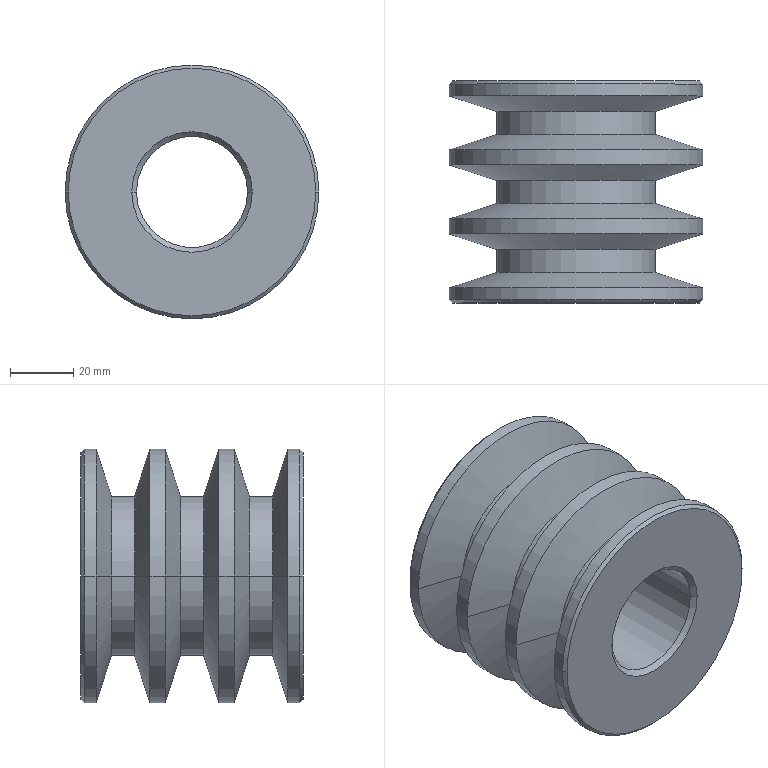Part | Creo | features DATUM PLANE 3, CHAMFER 2, COORDINATE SYSTEM 1, CURVE 1, PROTRUSION 1 | 1 solid | 38 faces | box 80 x 70 x 80 mm | volume 169146 mm3 | cone 20 | cylinder 16 | plane 2 | commonest cylinder face diameters 80 x8 50.008 x6 35 x2
STEP:
#1=CARTESIAN_POINT('',(0.,0.,0.));
#2=DIRECTION('',(0.,0.,1.));
#3=DIRECTION('',(1.,0.,0.));
#4=AXIS2_PLACEMENT_3D('',#1,#2,#3);
#5=CARTESIAN_POINT('',(39.,70.,0.));
#6=VERTEX_POINT('',#5);
#7=CARTESIAN_POINT('',(-39.,70.,0.));
#8=VERTEX_POINT('',#7);
#9=CARTESIAN_POINT('',(0.,70.,0.));
#10=DIRECTION('',(0.,1.,0.));
#11=DIRECTION('',(1.,0.,0.));
#12=AXIS2_PLACEMENT_3D('',#9,#10,#11);
#13=CIRCLE('',#12,39.);
#14=EDGE_CURVE('',#6,#8,#13,.T.);
#15=ORIENTED_EDGE('',*,*,#14,.F.);
#16=CARTESIAN_POINT('',(0.,70.,0.));
#17=DIRECTION('',(0.,1.,0.));
#18=DIRECTION('',(-1.,0.,0.));
#19=AXIS2_PLACEMENT_3D('',#16,#17,#18);
#20=CIRCLE('',#19,39.);
#21=EDGE_CURVE('',#8,#6,#20,.T.);
#22=ORIENTED_EDGE('',*,*,#21,.F.);
#23=EDGE_LOOP('',(#15,#22));
#24=FACE_OUTER_BOUND('',#23,.F.);
#25=CARTESIAN_POINT('',(-19.,70.,0.));
#26=VERTEX_POINT('',#25);
#27=CARTESIAN_POINT('',(19.,70.,0.));
#28=VERTEX_POINT('',#27);
#29=CARTESIAN_POINT('',(0.,70.,0.));
#30=DIRECTION('',(0.,1.,0.));
#31=DIRECTION('',(-1.,0.,0.));
#32=AXIS2_PLACEMENT_3D('',#29,#30,#31);
#33=CIRCLE('',#32,19.);
#34=EDGE_CURVE('',#26,#28,#33,.T.);
#35=ORIENTED_EDGE('',*,*,#34,.T.);
#36=CARTESIAN_POINT('',(0.,70.,0.));
#37=DIRECTION('',(0.,1.,0.));
#38=DIRECTION('',(1.,0.,0.));
#39=AXIS2_PLACEMENT_3D('',#36,#37,#38);
#40=CIRCLE('',#39,19.);
#41=EDGE_CURVE('',#28,#26,#40,.T.);
#42=ORIENTED_EDGE('',*,*,#41,.T.);
#43=EDGE_LOOP('',(#35,#42));
#44=FACE_BOUND('',#43,.F.);
#45=CARTESIAN_POINT('',(0.,70.,0.));
#46=DIRECTION('',(0.,1.,0.));
#47=DIRECTION('',(1.,0.,0.));
#48=AXIS2_PLACEMENT_3D('',#45,#46,#47);
#49=PLANE('',#48);
#50=ADVANCED_FACE('',(#24,#44),#49,.T.);
#51=CARTESIAN_POINT('',(-17.5,68.5,0.));
#52=VERTEX_POINT('',#51);
#53=CARTESIAN_POINT('',(17.5,68.5,0.));
#54=VERTEX_POINT('',#53);
#55=CARTESIAN_POINT('',(0.,68.5,0.));
#56=DIRECTION('',(0.,1.,0.));
#57=DIRECTION('',(-1.,0.,0.));
#58=AXIS2_PLACEMENT_3D('',#55,#56,#57);
#59=CIRCLE('',#58,17.5);
#60=EDGE_CURVE('',#52,#54,#59,.T.);
#61=ORIENTED_EDGE('',*,*,#60,.T.);
#62=CARTESIAN_POINT('',(17.5,68.5,0.000000002));
#63=DIRECTION('',(0.7071,0.7071,0.000000001));
#64=VECTOR('',#63,2.121);
#65=LINE('',#62,#64);
#66=EDGE_CURVE('',#54,#28,#65,.T.);
#67=ORIENTED_EDGE('',*,*,#66,.T.);
#68=ORIENTED_EDGE('',*,*,#34,.F.);
#69=CARTESIAN_POINT('',(-17.5,68.5,-0.000000002));
#70=DIRECTION('',(-0.7071,0.7071,-0.000000001));
#71=VECTOR('',#70,2.121);
#72=LINE('',#69,#71);
#73=EDGE_CURVE('',#52,#26,#72,.T.);
#74=ORIENTED_EDGE('',*,*,#73,.F.);
#75=EDGE_LOOP('',(#61,#67,#68,#74));
#76=FACE_OUTER_BOUND('',#75,.F.);
#77=CARTESIAN_POINT('',(0.,69.25,0.));
#78=DIRECTION('',(0.,1.,0.));
#79=DIRECTION('',(0.,0.,-1.));
#80=AXIS2_PLACEMENT_3D('',#77,#78,#79);
#81=CONICAL_SURFACE('',#80,18.25,45.);
#82=ADVANCED_FACE('',(#76),#81,.F.);
#83=ORIENTED_EDGE('',*,*,#60,.F.);
#84=CARTESIAN_POINT('',(-17.5,1.5,0.));
#85=VERTEX_POINT('',#84);
#86=CARTESIAN_POINT('',(-17.5,68.5,-0.000000002));
#87=DIRECTION('',(0.,-1.,0.));
#88=VECTOR('',#87,67.);
#89=LINE('',#86,#88);
#90=EDGE_CURVE('',#52,#85,#89,.T.);
#91=ORIENTED_EDGE('',*,*,#90,.T.);
#92=CARTESIAN_POINT('',(17.5,1.5,0.));
#93=VERTEX_POINT('',#92);
#94=CARTESIAN_POINT('',(0.,1.5,0.));
#95=DIRECTION('',(0.,1.,0.));
#96=DIRECTION('',(-1.,0.,0.));
#97=AXIS2_PLACEMENT_3D('',#94,#95,#96);
#98=CIRCLE('',#97,17.5);
#99=EDGE_CURVE('',#85,#93,#98,.T.);
#100=ORIENTED_EDGE('',*,*,#99,.T.);
#101=CARTESIAN_POINT('',(17.5,68.5,0.000000002));
#102=DIRECTION('',(0.,-1.,0.));
#103=VECTOR('',#102,67.);
#104=LINE('',#101,#103);
#105=EDGE_CURVE('',#54,#93,#104,.T.);
#106=ORIENTED_EDGE('',*,*,#105,.F.);
#107=EDGE_LOOP('',(#83,#91,#100,#106));
#108=FACE_OUTER_BOUND('',#107,.F.);
#109=CARTESIAN_POINT('',(0.,0.,0.));
#110=DIRECTION('',(0.,1.,0.));
#111=DIRECTION('',(1.,0.,0.));
#112=AXIS2_PLACEMENT_3D('',#109,#110,#111);
#113=CYLINDRICAL_SURFACE('',#112,17.5);
#114=ADVANCED_FACE('',(#108),#113,.F.);
#115=CARTESIAN_POINT('',(0.,68.5,0.));
#116=DIRECTION('',(0.,1.,0.));
#117=DIRECTION('',(1.,0.,0.));
#118=AXIS2_PLACEMENT_3D('',#115,#116,#117);
#119=CIRCLE('',#118,17.5);
#120=EDGE_CURVE('',#54,#52,#119,.T.);
#121=ORIENTED_EDGE('',*,*,#120,.F.);
#122=ORIENTED_EDGE('',*,*,#105,.T.);
#123=CARTESIAN_POINT('',(0.,1.5,0.));
#124=DIRECTION('',(0.,1.,0.));
#125=DIRECTION('',(1.,0.,0.));
#126=AXIS2_PLACEMENT_3D('',#123,#124,#125);
#127=CIRCLE('',#126,17.5);
#128=EDGE_CURVE('',#93,#85,#127,.T.);
#129=ORIENTED_EDGE('',*,*,#128,.T.);
#130=ORIENTED_EDGE('',*,*,#90,.F.);
#131=EDGE_LOOP('',(#121,#122,#129,#130));
#132=FACE_OUTER_BOUND('',#131,.F.);
#133=CARTESIAN_POINT('',(0.,0.,0.));
#134=DIRECTION('',(0.,1.,0.));
#135=DIRECTION('',(1.,0.,0.));
#136=AXIS2_PLACEMENT_3D('',#133,#134,#135);
#137=CYLINDRICAL_SURFACE('',#136,17.5);
#138=ADVANCED_FACE('',(#132),#137,.F.);
#139=ORIENTED_EDGE('',*,*,#120,.T.);
#140=ORIENTED_EDGE('',*,*,#73,.T.);
#141=ORIENTED_EDGE('',*,*,#41,.F.);
#142=ORIENTED_EDGE('',*,*,#66,.F.);
#143=EDGE_LOOP('',(#139,#140,#141,#142));
#144=FACE_OUTER_BOUND('',#143,.F.);
#145=CARTESIAN_POINT('',(0.,69.25,0.));
#146=DIRECTION('',(0.,1.,0.));
#147=DIRECTION('',(0.,0.,-1.));
#148=AXIS2_PLACEMENT_3D('',#145,#146,#147);
#149=CONICAL_SURFACE('',#148,18.25,45.);
#150=ADVANCED_FACE('',(#144),#149,.F.);
#151=CARTESIAN_POINT('',(19.,0.,0.));
#152=VERTEX_POINT('',#151);
#153=CARTESIAN_POINT('',(-19.,0.,0.));
#154=VERTEX_POINT('',#153);
#155=CARTESIAN_POINT('',(0.,0.,0.));
#156=DIRECTION('',(0.,1.,0.));
#157=DIRECTION('',(1.,0.,0.));
#158=AXIS2_PLACEMENT_3D('',#155,#156,#157);
#159=CIRCLE('',#158,19.);
#160=EDGE_CURVE('',#152,#154,#159,.T.);
#161=ORIENTED_EDGE('',*,*,#160,.T.);
#162=CARTESIAN_POINT('',(-19.,0.000000002,0.000000012));
#163=DIRECTION('',(0.7071,0.7071,-0.000000002));
#164=VECTOR('',#163,2.121);
#165=LINE('',#162,#164);
#166=EDGE_CURVE('',#154,#85,#165,.T.);
#167=ORIENTED_EDGE('',*,*,#166,.T.);
#168=ORIENTED_EDGE('',*,*,#128,.F.);
#169=CARTESIAN_POINT('',(19.,0.000000002,-0.000000012));
#170=DIRECTION('',(-0.7071,0.7071,0.000000002));
#171=VECTOR('',#170,2.121);
#172=LINE('',#169,#171);
#173=EDGE_CURVE('',#152,#93,#172,.T.);
#174=ORIENTED_EDGE('',*,*,#173,.F.);
#175=EDGE_LOOP('',(#161,#167,#168,#174));
#176=FACE_OUTER_BOUND('',#175,.F.);
#177=CARTESIAN_POINT('',(0.,0.75,0.));
#178=DIRECTION('',(0.,-1.,0.));
#179=DIRECTION('',(0.,0.,-1.));
#180=AXIS2_PLACEMENT_3D('',#177,#178,#179);
#181=CONICAL_SURFACE('',#180,18.25,45.);
#182=ADVANCED_FACE('',(#176),#181,.F.);
#183=CARTESIAN_POINT('',(39.,0.,0.));
#184=VERTEX_POINT('',#183);
#185=CARTESIAN_POINT('',(-39.,0.,0.));
#186=VERTEX_POINT('',#185);
#187=CARTESIAN_POINT('',(0.,0.,0.));
#188=DIRECTION('',(0.,1.,0.));
#189=DIRECTION('',(1.,0.,0.));
#190=AXIS2_PLACEMENT_3D('',#187,#188,#189);
#191=CIRCLE('',#190,39.);
#192=EDGE_CURVE('',#184,#186,#191,.T.);
#193=ORIENTED_EDGE('',*,*,#192,.T.);
#194=CARTESIAN_POINT('',(0.,0.,0.));
#195=DIRECTION('',(0.,1.,0.));
#196=DIRECTION('',(-1.,0.,0.));
#197=AXIS2_PLACEMENT_3D('',#194,#195,#196);
#198=CIRCLE('',#197,39.);
#199=EDGE_CURVE('',#186,#184,#198,.T.);
#200=ORIENTED_EDGE('',*,*,#199,.T.);
#201=EDGE_LOOP('',(#193,#200));
#202=FACE_OUTER_BOUND('',#201,.F.);
#203=CARTESIAN_POINT('',(0.,0.,0.));
#204=DIRECTION('',(0.,1.,0.));
#205=DIRECTION('',(-1.,0.,0.));
#206=AXIS2_PLACEMENT_3D('',#203,#204,#205);
#207=CIRCLE('',#206,19.);
#208=EDGE_CURVE('',#154,#152,#207,.T.);
#209=ORIENTED_EDGE('',*,*,#208,.F.);
#210=ORIENTED_EDGE('',*,*,#160,.F.);
#211=EDGE_LOOP('',(#209,#210));
#212=FACE_BOUND('',#211,.F.);
#213=CARTESIAN_POINT('',(0.,0.,0.));
#214=DIRECTION('',(0.,1.,0.));
#215=DIRECTION('',(1.,0.,0.));
#216=AXIS2_PLACEMENT_3D('',#213,#214,#215);
#217=PLANE('',#216);
#218=ADVANCED_FACE('',(#202,#212),#217,.F.);
#219=ORIENTED_EDGE('',*,*,#208,.T.);
#220=ORIENTED_EDGE('',*,*,#173,.T.);
#221=ORIENTED_EDGE('',*,*,#99,.F.);
#222=ORIENTED_EDGE('',*,*,#166,.F.);
#223=EDGE_LOOP('',(#219,#220,#221,#222));
#224=FACE_OUTER_BOUND('',#223,.F.);
#225=CARTESIAN_POINT('',(0.,0.75,0.));
#226=DIRECTION('',(0.,-1.,0.));
#227=DIRECTION('',(0.,0.,-1.));
#228=AXIS2_PLACEMENT_3D('',#225,#226,#227);
#229=CONICAL_SURFACE('',#228,18.25,45.);
#230=ADVANCED_FACE('',(#224),#229,.F.);
#231=CARTESIAN_POINT('',(40.,1.,0.));
#232=VERTEX_POINT('',#231);
#233=CARTESIAN_POINT('',(-40.,1.,0.));
#234=VERTEX_POINT('',#233);
#235=CARTESIAN_POINT('',(0.,1.,0.));
#236=DIRECTION('',(0.,1.,0.));
#237=DIRECTION('',(1.,0.,0.));
#238=AXIS2_PLACEMENT_3D('',#235,#236,#237);
#239=CIRCLE('',#238,40.);
#240=EDGE_CURVE('',#232,#234,#239,.T.);
#241=ORIENTED_EDGE('',*,*,#240,.T.);
#242=CARTESIAN_POINT('',(-40.,1.,-0.000000001));
#243=DIRECTION('',(0.7071,-0.7071,0.));
#244=VECTOR('',#243,1.414);
#245=LINE('',#242,#244);
#246=EDGE_CURVE('',#234,#186,#245,.T.);
#247=ORIENTED_EDGE('',*,*,#246,.T.);
#248=ORIENTED_EDGE('',*,*,#192,.F.);
#249=CARTESIAN_POINT('',(40.,1.,0.000000001));
#250=DIRECTION('',(-0.7071,-0.7071,0.));
#251=VECTOR('',#250,1.414);
#252=LINE('',#249,#251);
#253=EDGE_CURVE('',#232,#184,#252,.T.);
#254=ORIENTED_EDGE('',*,*,#253,.F.);
#255=EDGE_LOOP('',(#241,#247,#248,#254));
#256=FACE_OUTER_BOUND('',#255,.F.);
#257=CARTESIAN_POINT('',(0.,0.5,0.));
#258=DIRECTION('',(0.,1.,0.));
#259=DIRECTION('',(0.,0.,-1.));
#260=AXIS2_PLACEMENT_3D('',#257,#258,#259);
#261=CONICAL_SURFACE('',#260,39.5,45.);
#262=ADVANCED_FACE('',(#256),#261,.T.);
#263=ORIENTED_EDGE('',*,*,#240,.F.);
#264=CARTESIAN_POINT('',(40.,4.751,0.));
#265=VERTEX_POINT('',#264);
#266=CARTESIAN_POINT('',(40.,1.,0.000000001));
#267=DIRECTION('',(0.,1.,0.));
#268=VECTOR('',#267,3.751);
#269=LINE('',#266,#268);
#270=EDGE_CURVE('',#232,#265,#269,.T.);
#271=ORIENTED_EDGE('',*,*,#270,.T.);
#272=CARTESIAN_POINT('',(-40.,4.751,0.));
#273=VERTEX_POINT('',#272);
#274=CARTESIAN_POINT('',(0.,4.751,0.));
#275=DIRECTION('',(0.,1.,0.));
#276=DIRECTION('',(1.,0.,0.));
#277=AXIS2_PLACEMENT_3D('',#274,#275,#276);
#278=CIRCLE('',#277,40.);
#279=EDGE_CURVE('',#265,#273,#278,.T.);
#280=ORIENTED_EDGE('',*,*,#279,.T.);
#281=CARTESIAN_POINT('',(-40.,1.,-0.000000001));
#282=DIRECTION('',(0.,1.,0.));
#283=VECTOR('',#282,3.751);
#284=LINE('',#281,#283);
#285=EDGE_CURVE('',#234,#273,#284,.T.);
#286=ORIENTED_EDGE('',*,*,#285,.F.);
#287=EDGE_LOOP('',(#263,#271,#280,#286));
#288=FACE_OUTER_BOUND('',#287,.F.);
#289=CARTESIAN_POINT('',(0.,0.,0.));
#290=DIRECTION('',(0.,1.,0.));
#291=DIRECTION('',(1.,0.,0.));
#292=AXIS2_PLACEMENT_3D('',#289,#290,#291);
#293=CYLINDRICAL_SURFACE('',#292,40.);
#294=ADVANCED_FACE('',(#288),#293,.T.);
#295=CARTESIAN_POINT('',(0.,1.,0.));
#296=DIRECTION('',(0.,1.,0.));
#297=DIRECTION('',(-1.,0.,0.));
#298=AXIS2_PLACEMENT_3D('',#295,#296,#297);
#299=CIRCLE('',#298,40.);
#300=EDGE_CURVE('',#234,#232,#299,.T.);
#301=ORIENTED_EDGE('',*,*,#300,.F.);
#302=ORIENTED_EDGE('',*,*,#285,.T.);
#303=CARTESIAN_POINT('',(0.,4.751,0.));
#304=DIRECTION('',(0.,-1.,0.));
#305=DIRECTION('',(1.,0.,0.));
#306=AXIS2_PLACEMENT_3D('',#303,#304,#305);
#307=CIRCLE('',#306,40.);
#308=EDGE_CURVE('',#265,#273,#307,.T.);
#309=ORIENTED_EDGE('',*,*,#308,.F.);
#310=ORIENTED_EDGE('',*,*,#270,.F.);
#311=EDGE_LOOP('',(#301,#302,#309,#310));
#312=FACE_OUTER_BOUND('',#311,.F.);
#313=CARTESIAN_POINT('',(0.,0.,0.));
#314=DIRECTION('',(0.,1.,0.));
#315=DIRECTION('',(1.,0.,0.));
#316=AXIS2_PLACEMENT_3D('',#313,#314,#315);
#317=CYLINDRICAL_SURFACE('',#316,40.);
#318=ADVANCED_FACE('',(#312),#317,.T.);
#319=ORIENTED_EDGE('',*,*,#300,.T.);
#320=ORIENTED_EDGE('',*,*,#253,.T.);
#321=ORIENTED_EDGE('',*,*,#199,.F.);
#322=ORIENTED_EDGE('',*,*,#246,.F.);
#323=EDGE_LOOP('',(#319,#320,#321,#322));
#324=FACE_OUTER_BOUND('',#323,.F.);
#325=CARTESIAN_POINT('',(0.,0.5,0.));
#326=DIRECTION('',(0.,1.,0.));
#327=DIRECTION('',(0.,0.,-1.));
#328=AXIS2_PLACEMENT_3D('',#325,#326,#327);
#329=CONICAL_SURFACE('',#328,39.5,45.);
#330=ADVANCED_FACE('',(#324),#329,.T.);
#331=CARTESIAN_POINT('',(25.004,9.624,0.));
#332=VERTEX_POINT('',#331);
#333=CARTESIAN_POINT('',(40.,4.751,0.));
#334=DIRECTION('',(-0.9511,0.309,0.));
#335=VECTOR('',#334,15.768);
#336=LINE('',#333,#335);
#337=EDGE_CURVE('',#265,#332,#336,.T.);
#338=ORIENTED_EDGE('',*,*,#337,.F.);
#339=ORIENTED_EDGE('',*,*,#308,.T.);
#340=CARTESIAN_POINT('',(-25.004,9.624,0.));
#341=VERTEX_POINT('',#340);
#342=CARTESIAN_POINT('',(-40.,4.751,0.));
#343=DIRECTION('',(0.9511,0.309,0.));
#344=VECTOR('',#343,15.768);
#345=LINE('',#342,#344);
#346=EDGE_CURVE('',#273,#341,#345,.T.);
#347=ORIENTED_EDGE('',*,*,#346,.T.);
#348=CARTESIAN_POINT('',(0.,9.624,0.));
#349=DIRECTION('',(0.,-1.,0.));
#350=DIRECTION('',(1.,0.,0.));
#351=AXIS2_PLACEMENT_3D('',#348,#349,#350);
#352=CIRCLE('',#351,25.004);
#353=EDGE_CURVE('',#332,#341,#352,.T.);
#354=ORIENTED_EDGE('',*,*,#353,.F.);
#355=EDGE_LOOP('',(#338,#339,#347,#354));
#356=FACE_OUTER_BOUND('',#355,.F.);
#357=CARTESIAN_POINT('',(0.,7.188,0.));
#358=DIRECTION('',(0.,-1.,0.));
#359=DIRECTION('',(-1.,0.,0.));
#360=AXIS2_PLACEMENT_3D('',#357,#358,#359);
#361=CONICAL_SURFACE('',#360,32.502,72.);
#362=ADVANCED_FACE('',(#356),#361,.T.);
#363=ORIENTED_EDGE('',*,*,#337,.T.);
#364=CARTESIAN_POINT('',(0.,9.624,0.));
#365=DIRECTION('',(0.,1.,0.));
#366=DIRECTION('',(1.,0.,0.));
#367=AXIS2_PLACEMENT_3D('',#364,#365,#366);
#368=CIRCLE('',#367,25.004);
#369=EDGE_CURVE('',#332,#341,#368,.T.);
#370=ORIENTED_EDGE('',*,*,#369,.T.);
#371=ORIENTED_EDGE('',*,*,#346,.F.);
#372=ORIENTED_EDGE('',*,*,#279,.F.);
#373=EDGE_LOOP('',(#363,#370,#371,#372));
#374=FACE_OUTER_BOUND('',#373,.F.);
#375=CARTESIAN_POINT('',(0.,7.188,0.));
#376=DIRECTION('',(0.,-1.,0.));
#377=DIRECTION('',(-1.,0.,0.));
#378=AXIS2_PLACEMENT_3D('',#375,#376,#377);
#379=CONICAL_SURFACE('',#378,32.502,72.);
#380=ADVANCED_FACE('',(#374),#379,.T.);
#381=CARTESIAN_POINT('',(25.004,16.879,0.));
#382=VERTEX_POINT('',#381);
#383=CARTESIAN_POINT('',(25.004,9.624,0.));
#384=DIRECTION('',(0.,1.,0.));
#385=VECTOR('',#384,7.255);
#386=LINE('',#383,#385);
#387=EDGE_CURVE('',#332,#382,#386,.T.);
#388=ORIENTED_EDGE('',*,*,#387,.T.);
#389=CARTESIAN_POINT('',(-25.004,16.879,0.));
#390=VERTEX_POINT('',#389);
#391=CARTESIAN_POINT('',(0.,16.879,0.));
#392=DIRECTION('',(0.,1.,0.));
#393=DIRECTION('',(1.,0.,0.));
#394=AXIS2_PLACEMENT_3D('',#391,#392,#393);
#395=CIRCLE('',#394,25.004);
#396=EDGE_CURVE('',#382,#390,#395,.T.);
#397=ORIENTED_EDGE('',*,*,#396,.T.);
#398=CARTESIAN_POINT('',(-25.004,9.624,0.));
#399=DIRECTION('',(0.,1.,0.));
#400=VECTOR('',#399,7.255);
#401=LINE('',#398,#400);
#402=EDGE_CURVE('',#341,#390,#401,.T.);
#403=ORIENTED_EDGE('',*,*,#402,.F.);
#404=ORIENTED_EDGE('',*,*,#369,.F.);
#405=EDGE_LOOP('',(#388,#397,#403,#404));
#406=FACE_OUTER_BOUND('',#405,.F.);
#407=CARTESIAN_POINT('',(0.,0.,0.));
#408=DIRECTION('',(0.,1.,0.));
#409=DIRECTION('',(1.,0.,0.));
#410=AXIS2_PLACEMENT_3D('',#407,#408,#409);
#411=CYLINDRICAL_SURFACE('',#410,25.004);
#412=ADVANCED_FACE('',(#406),#411,.T.);
#413=ORIENTED_EDGE('',*,*,#387,.F.);
#414=ORIENTED_EDGE('',*,*,#353,.T.);
#415=ORIENTED_EDGE('',*,*,#402,.T.);
#416=CARTESIAN_POINT('',(0.,16.879,0.));
#417=DIRECTION('',(0.,-1.,0.));
#418=DIRECTION('',(1.,0.,0.));
#419=AXIS2_PLACEMENT_3D('',#416,#417,#418);
#420=CIRCLE('',#419,25.004);
#421=EDGE_CURVE('',#382,#390,#420,.T.);
#422=ORIENTED_EDGE('',*,*,#421,.F.);
#423=EDGE_LOOP('',(#413,#414,#415,#422));
#424=FACE_OUTER_BOUND('',#423,.F.);
#425=CARTESIAN_POINT('',(0.,0.,0.));
#426=DIRECTION('',(0.,1.,0.));
#427=DIRECTION('',(1.,0.,0.));
#428=AXIS2_PLACEMENT_3D('',#425,#426,#427);
#429=CYLINDRICAL_SURFACE('',#428,25.004);
#430=ADVANCED_FACE('',(#424),#429,.T.);
#431=CARTESIAN_POINT('',(40.,21.751,0.));
#432=VERTEX_POINT('',#431);
#433=CARTESIAN_POINT('',(25.004,16.879,0.));
#434=DIRECTION('',(0.9511,0.309,0.));
#435=VECTOR('',#434,15.768);
#436=LINE('',#433,#435);
#437=EDGE_CURVE('',#382,#432,#436,.T.);
#438=ORIENTED_EDGE('',*,*,#437,.F.);
#439=ORIENTED_EDGE('',*,*,#421,.T.);
#440=CARTESIAN_POINT('',(-40.,21.751,0.));
#441=VERTEX_POINT('',#440);
#442=CARTESIAN_POINT('',(-25.004,16.879,0.));
#443=DIRECTION('',(-0.9511,0.309,0.));
#444=VECTOR('',#443,15.768);
#445=LINE('',#442,#444);
#446=EDGE_CURVE('',#390,#441,#445,.T.);
#447=ORIENTED_EDGE('',*,*,#446,.T.);
#448=CARTESIAN_POINT('',(0.,21.751,0.));
#449=DIRECTION('',(0.,-1.,0.));
#450=DIRECTION('',(1.,0.,0.));
#451=AXIS2_PLACEMENT_3D('',#448,#449,#450);
#452=CIRCLE('',#451,40.);
#453=EDGE_CURVE('',#432,#441,#452,.T.);
#454=ORIENTED_EDGE('',*,*,#453,.F.);
#455=EDGE_LOOP('',(#438,#439,#447,#454));
#456=FACE_OUTER_BOUND('',#455,.F.);
#457=CARTESIAN_POINT('',(0.,19.315,0.));
#458=DIRECTION('',(0.,1.,0.));
#459=DIRECTION('',(1.,0.,0.));
#460=AXIS2_PLACEMENT_3D('',#457,#458,#459);
#461=CONICAL_SURFACE('',#460,32.502,72.);
#462=ADVANCED_FACE('',(#456),#461,.T.);
#463=ORIENTED_EDGE('',*,*,#437,.T.);
#464=CARTESIAN_POINT('',(0.,21.751,0.));
#465=DIRECTION('',(0.,1.,0.));
#466=DIRECTION('',(1.,0.,0.));
#467=AXIS2_PLACEMENT_3D('',#464,#465,#466);
#468=CIRCLE('',#467,40.);
#469=EDGE_CURVE('',#432,#441,#468,.T.);
#470=ORIENTED_EDGE('',*,*,#469,.T.);
#471=ORIENTED_EDGE('',*,*,#446,.F.);
#472=ORIENTED_EDGE('',*,*,#396,.F.);
#473=EDGE_LOOP('',(#463,#470,#471,#472));
#474=FACE_OUTER_BOUND('',#473,.F.);
#475=CARTESIAN_POINT('',(0.,19.315,0.));
#476=DIRECTION('',(0.,1.,0.));
#477=DIRECTION('',(1.,0.,0.));
#478=AXIS2_PLACEMENT_3D('',#475,#476,#477);
#479=CONICAL_SURFACE('',#478,32.502,72.);
#480=ADVANCED_FACE('',(#474),#479,.T.);
#481=CARTESIAN_POINT('',(40.,26.497,0.));
#482=VERTEX_POINT('',#481);
#483=CARTESIAN_POINT('',(40.,21.751,0.));
#484=DIRECTION('',(0.,1.,0.));
#485=VECTOR('',#484,4.746);
#486=LINE('',#483,#485);
#487=EDGE_CURVE('',#432,#482,#486,.T.);
#488=ORIENTED_EDGE('',*,*,#487,.T.);
#489=CARTESIAN_POINT('',(-40.,26.497,0.));
#490=VERTEX_POINT('',#489);
#491=CARTESIAN_POINT('',(0.,26.497,0.));
#492=DIRECTION('',(0.,1.,0.));
#493=DIRECTION('',(1.,0.,0.));
#494=AXIS2_PLACEMENT_3D('',#491,#492,#493);
#495=CIRCLE('',#494,40.);
#496=EDGE_CURVE('',#482,#490,#495,.T.);
#497=ORIENTED_EDGE('',*,*,#496,.T.);
#498=CARTESIAN_POINT('',(-40.,21.751,0.));
#499=DIRECTION('',(0.,1.,0.));
#500=VECTOR('',#499,4.746);
#501=LINE('',#498,#500);
#502=EDGE_CURVE('',#441,#490,#501,.T.);
#503=ORIENTED_EDGE('',*,*,#502,.F.);
#504=ORIENTED_EDGE('',*,*,#469,.F.);
#505=EDGE_LOOP('',(#488,#497,#503,#504));
#506=FACE_OUTER_BOUND('',#505,.F.);
#507=CARTESIAN_POINT('',(0.,0.,0.));
#508=DIRECTION('',(0.,1.,0.));
#509=DIRECTION('',(1.,0.,0.));
#510=AXIS2_PLACEMENT_3D('',#507,#508,#509);
#511=CYLINDRICAL_SURFACE('',#510,40.);
#512=ADVANCED_FACE('',(#506),#511,.T.);
#513=ORIENTED_EDGE('',*,*,#487,.F.);
#514=ORIENTED_EDGE('',*,*,#453,.T.);
#515=ORIENTED_EDGE('',*,*,#502,.T.);
#516=CARTESIAN_POINT('',(0.,26.497,0.));
#517=DIRECTION('',(0.,-1.,0.));
#518=DIRECTION('',(1.,0.,0.));
#519=AXIS2_PLACEMENT_3D('',#516,#517,#518);
#520=CIRCLE('',#519,40.);
#521=EDGE_CURVE('',#482,#490,#520,.T.);
#522=ORIENTED_EDGE('',*,*,#521,.F.);
#523=EDGE_LOOP('',(#513,#514,#515,#522));
#524=FACE_OUTER_BOUND('',#523,.F.);
#525=CARTESIAN_POINT('',(0.,0.,0.));
#526=DIRECTION('',(0.,1.,0.));
#527=DIRECTION('',(1.,0.,0.));
#528=AXIS2_PLACEMENT_3D('',#525,#526,#527);
#529=CYLINDRICAL_SURFACE('',#528,40.);
#530=ADVANCED_FACE('',(#524),#529,.T.);
#531=CARTESIAN_POINT('',(25.004,31.369,0.));
#532=VERTEX_POINT('',#531);
#533=CARTESIAN_POINT('',(40.,26.497,0.));
#534=DIRECTION('',(-0.9511,0.309,0.));
#535=VECTOR('',#534,15.768);
#536=LINE('',#533,#535);
#537=EDGE_CURVE('',#482,#532,#536,.T.);
#538=ORIENTED_EDGE('',*,*,#537,.F.);
#539=ORIENTED_EDGE('',*,*,#521,.T.);
#540=CARTESIAN_POINT('',(-25.004,31.369,0.));
#541=VERTEX_POINT('',#540);
#542=CARTESIAN_POINT('',(-40.,26.497,0.));
#543=DIRECTION('',(0.9511,0.309,0.));
#544=VECTOR('',#543,15.768);
#545=LINE('',#542,#544);
#546=EDGE_CURVE('',#490,#541,#545,.T.);
#547=ORIENTED_EDGE('',*,*,#546,.T.);
#548=CARTESIAN_POINT('',(0.,31.369,0.));
#549=DIRECTION('',(0.,-1.,0.));
#550=DIRECTION('',(1.,0.,0.));
#551=AXIS2_PLACEMENT_3D('',#548,#549,#550);
#552=CIRCLE('',#551,25.004);
#553=EDGE_CURVE('',#532,#541,#552,.T.);
#554=ORIENTED_EDGE('',*,*,#553,.F.);
#555=EDGE_LOOP('',(#538,#539,#547,#554));
#556=FACE_OUTER_BOUND('',#555,.F.);
#557=CARTESIAN_POINT('',(0.,28.933,0.));
#558=DIRECTION('',(0.,-1.,0.));
#559=DIRECTION('',(-1.,0.,0.));
#560=AXIS2_PLACEMENT_3D('',#557,#558,#559);
#561=CONICAL_SURFACE('',#560,32.502,72.);
#562=ADVANCED_FACE('',(#556),#561,.T.);
#563=ORIENTED_EDGE('',*,*,#537,.T.);
#564=CARTESIAN_POINT('',(0.,31.369,0.));
#565=DIRECTION('',(0.,1.,0.));
#566=DIRECTION('',(1.,0.,0.));
#567=AXIS2_PLACEMENT_3D('',#564,#565,#566);
#568=CIRCLE('',#567,25.004);
#569=EDGE_CURVE('',#532,#541,#568,.T.);
#570=ORIENTED_EDGE('',*,*,#569,.T.);
#571=ORIENTED_EDGE('',*,*,#546,.F.);
#572=ORIENTED_EDGE('',*,*,#496,.F.);
#573=EDGE_LOOP('',(#563,#570,#571,#572));
#574=FACE_OUTER_BOUND('',#573,.F.);
#575=CARTESIAN_POINT('',(0.,28.933,0.));
#576=DIRECTION('',(0.,-1.,0.));
#577=DIRECTION('',(-1.,0.,0.));
#578=AXIS2_PLACEMENT_3D('',#575,#576,#577);
#579=CONICAL_SURFACE('',#578,32.502,72.);
#580=ADVANCED_FACE('',(#574),#579,.T.);
#581=CARTESIAN_POINT('',(25.004,38.624,0.));
#582=VERTEX_POINT('',#581);
#583=CARTESIAN_POINT('',(25.004,31.369,0.));
#584=DIRECTION('',(0.,1.,0.));
#585=VECTOR('',#584,7.255);
#586=LINE('',#583,#585);
#587=EDGE_CURVE('',#532,#582,#586,.T.);
#588=ORIENTED_EDGE('',*,*,#587,.T.);
#589=CARTESIAN_POINT('',(-25.004,38.624,0.));
#590=VERTEX_POINT('',#589);
#591=CARTESIAN_POINT('',(0.,38.624,0.));
#592=DIRECTION('',(0.,1.,0.));
#593=DIRECTION('',(1.,0.,0.));
#594=AXIS2_PLACEMENT_3D('',#591,#592,#593);
#595=CIRCLE('',#594,25.004);
#596=EDGE_CURVE('',#582,#590,#595,.T.);
#597=ORIENTED_EDGE('',*,*,#596,.T.);
#598=CARTESIAN_POINT('',(-25.004,31.369,0.));
#599=DIRECTION('',(0.,1.,0.));
#600=VECTOR('',#599,7.255);
#601=LINE('',#598,#600);
#602=EDGE_CURVE('',#541,#590,#601,.T.);
#603=ORIENTED_EDGE('',*,*,#602,.F.);
#604=ORIENTED_EDGE('',*,*,#569,.F.);
#605=EDGE_LOOP('',(#588,#597,#603,#604));
#606=FACE_OUTER_BOUND('',#605,.F.);
#607=CARTESIAN_POINT('',(0.,0.,0.));
#608=DIRECTION('',(0.,1.,0.));
#609=DIRECTION('',(1.,0.,0.));
#610=AXIS2_PLACEMENT_3D('',#607,#608,#609);
#611=CYLINDRICAL_SURFACE('',#610,25.004);
#612=ADVANCED_FACE('',(#606),#611,.T.);
#613=ORIENTED_EDGE('',*,*,#587,.F.);
#614=ORIENTED_EDGE('',*,*,#553,.T.);
#615=ORIENTED_EDGE('',*,*,#602,.T.);
#616=CARTESIAN_POINT('',(0.,38.624,0.));
#617=DIRECTION('',(0.,-1.,0.));
#618=DIRECTION('',(1.,0.,0.));
#619=AXIS2_PLACEMENT_3D('',#616,#617,#618);
#620=CIRCLE('',#619,25.004);
#621=EDGE_CURVE('',#582,#590,#620,.T.);
#622=ORIENTED_EDGE('',*,*,#621,.F.);
#623=EDGE_LOOP('',(#613,#614,#615,#622));
#624=FACE_OUTER_BOUND('',#623,.F.);
#625=CARTESIAN_POINT('',(0.,0.,0.));
#626=DIRECTION('',(0.,1.,0.));
#627=DIRECTION('',(1.,0.,0.));
#628=AXIS2_PLACEMENT_3D('',#625,#626,#627);
#629=CYLINDRICAL_SURFACE('',#628,25.004);
#630=ADVANCED_FACE('',(#624),#629,.T.);
#631=CARTESIAN_POINT('',(40.,43.497,0.));
#632=VERTEX_POINT('',#631);
#633=CARTESIAN_POINT('',(25.004,38.624,0.));
#634=DIRECTION('',(0.9511,0.309,0.));
#635=VECTOR('',#634,15.768);
#636=LINE('',#633,#635);
#637=EDGE_CURVE('',#582,#632,#636,.T.);
#638=ORIENTED_EDGE('',*,*,#637,.F.);
#639=ORIENTED_EDGE('',*,*,#621,.T.);
#640=CARTESIAN_POINT('',(-40.,43.497,0.));
#641=VERTEX_POINT('',#640);
#642=CARTESIAN_POINT('',(-25.004,38.624,0.));
#643=DIRECTION('',(-0.9511,0.309,0.));
#644=VECTOR('',#643,15.768);
#645=LINE('',#642,#644);
#646=EDGE_CURVE('',#590,#641,#645,.T.);
#647=ORIENTED_EDGE('',*,*,#646,.T.);
#648=CARTESIAN_POINT('',(0.,43.497,0.));
#649=DIRECTION('',(0.,-1.,0.));
#650=DIRECTION('',(1.,0.,0.));
#651=AXIS2_PLACEMENT_3D('',#648,#649,#650);
#652=CIRCLE('',#651,40.);
#653=EDGE_CURVE('',#632,#641,#652,.T.);
#654=ORIENTED_EDGE('',*,*,#653,.F.);
#655=EDGE_LOOP('',(#638,#639,#647,#654));
#656=FACE_OUTER_BOUND('',#655,.F.);
#657=CARTESIAN_POINT('',(0.,41.061,0.));
#658=DIRECTION('',(0.,1.,0.));
#659=DIRECTION('',(1.,0.,0.));
#660=AXIS2_PLACEMENT_3D('',#657,#658,#659);
#661=CONICAL_SURFACE('',#660,32.502,72.);
#662=ADVANCED_FACE('',(#656),#661,.T.);
#663=ORIENTED_EDGE('',*,*,#637,.T.);
#664=CARTESIAN_POINT('',(0.,43.497,0.));
#665=DIRECTION('',(0.,1.,0.));
#666=DIRECTION('',(1.,0.,0.));
#667=AXIS2_PLACEMENT_3D('',#664,#665,#666);
#668=CIRCLE('',#667,40.);
#669=EDGE_CURVE('',#632,#641,#668,.T.);
#670=ORIENTED_EDGE('',*,*,#669,.T.);
#671=ORIENTED_EDGE('',*,*,#646,.F.);
#672=ORIENTED_EDGE('',*,*,#596,.F.);
#673=EDGE_LOOP('',(#663,#670,#671,#672));
#674=FACE_OUTER_BOUND('',#673,.F.);
#675=CARTESIAN_POINT('',(0.,41.061,0.));
#676=DIRECTION('',(0.,1.,0.));
#677=DIRECTION('',(1.,0.,0.));
#678=AXIS2_PLACEMENT_3D('',#675,#676,#677);
#679=CONICAL_SURFACE('',#678,32.502,72.);
#680=ADVANCED_FACE('',(#674),#679,.T.);
#681=CARTESIAN_POINT('',(40.,48.242,0.));
#682=VERTEX_POINT('',#681);
#683=CARTESIAN_POINT('',(40.,43.497,0.));
#684=DIRECTION('',(0.,1.,0.));
#685=VECTOR('',#684,4.746);
#686=LINE('',#683,#685);
#687=EDGE_CURVE('',#632,#682,#686,.T.);
#688=ORIENTED_EDGE('',*,*,#687,.T.);
#689=CARTESIAN_POINT('',(-40.,48.242,0.));
#690=VERTEX_POINT('',#689);
#691=CARTESIAN_POINT('',(0.,48.242,0.));
#692=DIRECTION('',(0.,1.,0.));
#693=DIRECTION('',(1.,0.,0.));
#694=AXIS2_PLACEMENT_3D('',#691,#692,#693);
#695=CIRCLE('',#694,40.);
#696=EDGE_CURVE('',#682,#690,#695,.T.);
#697=ORIENTED_EDGE('',*,*,#696,.T.);
#698=CARTESIAN_POINT('',(-40.,43.497,0.));
#699=DIRECTION('',(0.,1.,0.));
#700=VECTOR('',#699,4.746);
#701=LINE('',#698,#700);
#702=EDGE_CURVE('',#641,#690,#701,.T.);
#703=ORIENTED_EDGE('',*,*,#702,.F.);
#704=ORIENTED_EDGE('',*,*,#669,.F.);
#705=EDGE_LOOP('',(#688,#697,#703,#704));
#706=FACE_OUTER_BOUND('',#705,.F.);
#707=CARTESIAN_POINT('',(0.,0.,0.));
#708=DIRECTION('',(0.,1.,0.));
#709=DIRECTION('',(1.,0.,0.));
#710=AXIS2_PLACEMENT_3D('',#707,#708,#709);
#711=CYLINDRICAL_SURFACE('',#710,40.);
#712=ADVANCED_FACE('',(#706),#711,.T.);
#713=ORIENTED_EDGE('',*,*,#687,.F.);
#714=ORIENTED_EDGE('',*,*,#653,.T.);
#715=ORIENTED_EDGE('',*,*,#702,.T.);
#716=CARTESIAN_POINT('',(0.,48.242,0.));
#717=DIRECTION('',(0.,-1.,0.));
#718=DIRECTION('',(1.,0.,0.));
#719=AXIS2_PLACEMENT_3D('',#716,#717,#718);
#720=CIRCLE('',#719,40.);
#721=EDGE_CURVE('',#682,#690,#720,.T.);
#722=ORIENTED_EDGE('',*,*,#721,.F.);
#723=EDGE_LOOP('',(#713,#714,#715,#722));
#724=FACE_OUTER_BOUND('',#723,.F.);
#725=CARTESIAN_POINT('',(0.,0.,0.));
#726=DIRECTION('',(0.,1.,0.));
#727=DIRECTION('',(1.,0.,0.));
#728=AXIS2_PLACEMENT_3D('',#725,#726,#727);
#729=CYLINDRICAL_SURFACE('',#728,40.);
#730=ADVANCED_FACE('',(#724),#729,.T.);
#731=CARTESIAN_POINT('',(25.004,53.115,0.));
#732=VERTEX_POINT('',#731);
#733=CARTESIAN_POINT('',(40.,48.242,0.));
#734=DIRECTION('',(-0.9511,0.309,0.));
#735=VECTOR('',#734,15.768);
#736=LINE('',#733,#735);
#737=EDGE_CURVE('',#682,#732,#736,.T.);
#738=ORIENTED_EDGE('',*,*,#737,.F.);
#739=ORIENTED_EDGE('',*,*,#721,.T.);
#740=CARTESIAN_POINT('',(-25.004,53.115,0.));
#741=VERTEX_POINT('',#740);
#742=CARTESIAN_POINT('',(-40.,48.242,0.));
#743=DIRECTION('',(0.9511,0.309,0.));
#744=VECTOR('',#743,15.768);
#745=LINE('',#742,#744);
#746=EDGE_CURVE('',#690,#741,#745,.T.);
#747=ORIENTED_EDGE('',*,*,#746,.T.);
#748=CARTESIAN_POINT('',(0.,53.115,0.));
#749=DIRECTION('',(0.,-1.,0.));
#750=DIRECTION('',(1.,0.,0.));
#751=AXIS2_PLACEMENT_3D('',#748,#749,#750);
#752=CIRCLE('',#751,25.004);
#753=EDGE_CURVE('',#732,#741,#752,.T.);
#754=ORIENTED_EDGE('',*,*,#753,.F.);
#755=EDGE_LOOP('',(#738,#739,#747,#754));
#756=FACE_OUTER_BOUND('',#755,.F.);
#757=CARTESIAN_POINT('',(0.,50.679,0.));
#758=DIRECTION('',(0.,-1.,0.));
#759=DIRECTION('',(-1.,0.,0.));
#760=AXIS2_PLACEMENT_3D('',#757,#758,#759);
#761=CONICAL_SURFACE('',#760,32.502,72.);
#762=ADVANCED_FACE('',(#756),#761,.T.);
#763=ORIENTED_EDGE('',*,*,#737,.T.);
#764=CARTESIAN_POINT('',(0.,53.115,0.));
#765=DIRECTION('',(0.,1.,0.));
#766=DIRECTION('',(1.,0.,0.));
#767=AXIS2_PLACEMENT_3D('',#764,#765,#766);
#768=CIRCLE('',#767,25.004);
#769=EDGE_CURVE('',#732,#741,#768,.T.);
#770=ORIENTED_EDGE('',*,*,#769,.T.);
#771=ORIENTED_EDGE('',*,*,#746,.F.);
#772=ORIENTED_EDGE('',*,*,#696,.F.);
#773=EDGE_LOOP('',(#763,#770,#771,#772));
#774=FACE_OUTER_BOUND('',#773,.F.);
#775=CARTESIAN_POINT('',(0.,50.679,0.));
#776=DIRECTION('',(0.,-1.,0.));
#777=DIRECTION('',(-1.,0.,0.));
#778=AXIS2_PLACEMENT_3D('',#775,#776,#777);
#779=CONICAL_SURFACE('',#778,32.502,72.);
#780=ADVANCED_FACE('',(#774),#779,.T.);
#781=CARTESIAN_POINT('',(25.004,60.37,0.));
#782=VERTEX_POINT('',#781);
#783=CARTESIAN_POINT('',(25.004,53.115,0.));
#784=DIRECTION('',(0.,1.,0.));
#785=VECTOR('',#784,7.255);
#786=LINE('',#783,#785);
#787=EDGE_CURVE('',#732,#782,#786,.T.);
#788=ORIENTED_EDGE('',*,*,#787,.T.);
#789=CARTESIAN_POINT('',(-25.004,60.37,0.));
#790=VERTEX_POINT('',#789);
#791=CARTESIAN_POINT('',(0.,60.37,0.));
#792=DIRECTION('',(0.,1.,0.));
#793=DIRECTION('',(1.,0.,0.));
#794=AXIS2_PLACEMENT_3D('',#791,#792,#793);
#795=CIRCLE('',#794,25.004);
#796=EDGE_CURVE('',#782,#790,#795,.T.);
#797=ORIENTED_EDGE('',*,*,#796,.T.);
#798=CARTESIAN_POINT('',(-25.004,53.115,0.));
#799=DIRECTION('',(0.,1.,0.));
#800=VECTOR('',#799,7.255);
#801=LINE('',#798,#800);
#802=EDGE_CURVE('',#741,#790,#801,.T.);
#803=ORIENTED_EDGE('',*,*,#802,.F.);
#804=ORIENTED_EDGE('',*,*,#769,.F.);
#805=EDGE_LOOP('',(#788,#797,#803,#804));
#806=FACE_OUTER_BOUND('',#805,.F.);
#807=CARTESIAN_POINT('',(0.,0.,0.));
#808=DIRECTION('',(0.,1.,0.));
#809=DIRECTION('',(1.,0.,0.));
#810=AXIS2_PLACEMENT_3D('',#807,#808,#809);
#811=CYLINDRICAL_SURFACE('',#810,25.004);
#812=ADVANCED_FACE('',(#806),#811,.T.);
#813=ORIENTED_EDGE('',*,*,#787,.F.);
#814=ORIENTED_EDGE('',*,*,#753,.T.);
#815=ORIENTED_EDGE('',*,*,#802,.T.);
#816=CARTESIAN_POINT('',(0.,60.37,0.));
#817=DIRECTION('',(0.,-1.,0.));
#818=DIRECTION('',(1.,0.,0.));
#819=AXIS2_PLACEMENT_3D('',#816,#817,#818);
#820=CIRCLE('',#819,25.004);
#821=EDGE_CURVE('',#782,#790,#820,.T.);
#822=ORIENTED_EDGE('',*,*,#821,.F.);
#823=EDGE_LOOP('',(#813,#814,#815,#822));
#824=FACE_OUTER_BOUND('',#823,.F.);
#825=CARTESIAN_POINT('',(0.,0.,0.));
#826=DIRECTION('',(0.,1.,0.));
#827=DIRECTION('',(1.,0.,0.));
#828=AXIS2_PLACEMENT_3D('',#825,#826,#827);
#829=CYLINDRICAL_SURFACE('',#828,25.004);
#830=ADVANCED_FACE('',(#824),#829,.T.);
#831=CARTESIAN_POINT('',(40.,65.242,0.));
#832=VERTEX_POINT('',#831);
#833=CARTESIAN_POINT('',(25.004,60.37,0.));
#834=DIRECTION('',(0.9511,0.309,0.));
#835=VECTOR('',#834,15.768);
#836=LINE('',#833,#835);
#837=EDGE_CURVE('',#782,#832,#836,.T.);
#838=ORIENTED_EDGE('',*,*,#837,.F.);
#839=ORIENTED_EDGE('',*,*,#821,.T.);
#840=CARTESIAN_POINT('',(-40.,65.242,0.));
#841=VERTEX_POINT('',#840);
#842=CARTESIAN_POINT('',(-25.004,60.37,0.));
#843=DIRECTION('',(-0.9511,0.309,0.));
#844=VECTOR('',#843,15.768);
#845=LINE('',#842,#844);
#846=EDGE_CURVE('',#790,#841,#845,.T.);
#847=ORIENTED_EDGE('',*,*,#846,.T.);
#848=CARTESIAN_POINT('',(0.,65.242,0.));
#849=DIRECTION('',(0.,-1.,0.));
#850=DIRECTION('',(1.,0.,0.));
#851=AXIS2_PLACEMENT_3D('',#848,#849,#850);
#852=CIRCLE('',#851,40.);
#853=EDGE_CURVE('',#832,#841,#852,.T.);
#854=ORIENTED_EDGE('',*,*,#853,.F.);
#855=EDGE_LOOP('',(#838,#839,#847,#854));
#856=FACE_OUTER_BOUND('',#855,.F.);
#857=CARTESIAN_POINT('',(0.,62.806,0.));
#858=DIRECTION('',(0.,1.,0.));
#859=DIRECTION('',(1.,0.,0.));
#860=AXIS2_PLACEMENT_3D('',#857,#858,#859);
#861=CONICAL_SURFACE('',#860,32.502,72.);
#862=ADVANCED_FACE('',(#856),#861,.T.);
#863=ORIENTED_EDGE('',*,*,#837,.T.);
#864=CARTESIAN_POINT('',(0.,65.242,0.));
#865=DIRECTION('',(0.,1.,0.));
#866=DIRECTION('',(1.,0.,0.));
#867=AXIS2_PLACEMENT_3D('',#864,#865,#866);
#868=CIRCLE('',#867,40.);
#869=EDGE_CURVE('',#832,#841,#868,.T.);
#870=ORIENTED_EDGE('',*,*,#869,.T.);
#871=ORIENTED_EDGE('',*,*,#846,.F.);
#872=ORIENTED_EDGE('',*,*,#796,.F.);
#873=EDGE_LOOP('',(#863,#870,#871,#872));
#874=FACE_OUTER_BOUND('',#873,.F.);
#875=CARTESIAN_POINT('',(0.,62.806,0.));
#876=DIRECTION('',(0.,1.,0.));
#877=DIRECTION('',(1.,0.,0.));
#878=AXIS2_PLACEMENT_3D('',#875,#876,#877);
#879=CONICAL_SURFACE('',#878,32.502,72.);
#880=ADVANCED_FACE('',(#874),#879,.T.);
#881=CARTESIAN_POINT('',(40.,69.,0.));
#882=VERTEX_POINT('',#881);
#883=CARTESIAN_POINT('',(-40.,69.,0.));
#884=VERTEX_POINT('',#883);
#885=CARTESIAN_POINT('',(0.,69.,0.));
#886=DIRECTION('',(0.,1.,0.));
#887=DIRECTION('',(1.,0.,0.));
#888=AXIS2_PLACEMENT_3D('',#885,#886,#887);
#889=CIRCLE('',#888,40.);
#890=EDGE_CURVE('',#882,#884,#889,.T.);
#891=ORIENTED_EDGE('',*,*,#890,.T.);
#892=CARTESIAN_POINT('',(-40.,65.242,0.));
#893=DIRECTION('',(0.,1.,0.000000001));
#894=VECTOR('',#893,3.758);
#895=LINE('',#892,#894);
#896=EDGE_CURVE('',#841,#884,#895,.T.);
#897=ORIENTED_EDGE('',*,*,#896,.F.);
#898=ORIENTED_EDGE('',*,*,#869,.F.);
#899=CARTESIAN_POINT('',(40.,65.242,0.));
#900=DIRECTION('',(0.,1.,-0.000000001));
#901=VECTOR('',#900,3.758);
#902=LINE('',#899,#901);
#903=EDGE_CURVE('',#832,#882,#902,.T.);
#904=ORIENTED_EDGE('',*,*,#903,.T.);
#905=EDGE_LOOP('',(#891,#897,#898,#904));
#906=FACE_OUTER_BOUND('',#905,.F.);
#907=CARTESIAN_POINT('',(0.,0.,0.));
#908=DIRECTION('',(0.,1.,0.));
#909=DIRECTION('',(1.,0.,0.));
#910=AXIS2_PLACEMENT_3D('',#907,#908,#909);
#911=CYLINDRICAL_SURFACE('',#910,40.);
#912=ADVANCED_FACE('',(#906),#911,.T.);
#913=ORIENTED_EDGE('',*,*,#14,.T.);
#914=CARTESIAN_POINT('',(-39.,70.,0.000000006));
#915=DIRECTION('',(-0.7071,-0.7071,-0.000000001));
#916=VECTOR('',#915,1.414);
#917=LINE('',#914,#916);
#918=EDGE_CURVE('',#8,#884,#917,.T.);
#919=ORIENTED_EDGE('',*,*,#918,.T.);
#920=ORIENTED_EDGE('',*,*,#890,.F.);
#921=CARTESIAN_POINT('',(39.,70.,-0.000000006));
#922=DIRECTION('',(0.7071,-0.7071,0.000000001));
#923=VECTOR('',#922,1.414);
#924=LINE('',#921,#923);
#925=EDGE_CURVE('',#6,#882,#924,.T.);
#926=ORIENTED_EDGE('',*,*,#925,.F.);
#927=EDGE_LOOP('',(#913,#919,#920,#926));
#928=FACE_OUTER_BOUND('',#927,.F.);
#929=CARTESIAN_POINT('',(0.,69.5,0.));
#930=DIRECTION('',(0.,-1.,0.));
#931=DIRECTION('',(0.,0.,-1.));
#932=AXIS2_PLACEMENT_3D('',#929,#930,#931);
#933=CONICAL_SURFACE('',#932,39.5,45.);
#934=ADVANCED_FACE('',(#928),#933,.T.);
#935=ORIENTED_EDGE('',*,*,#21,.T.);
#936=ORIENTED_EDGE('',*,*,#925,.T.);
#937=CARTESIAN_POINT('',(0.,69.,0.));
#938=DIRECTION('',(0.,1.,0.));
#939=DIRECTION('',(-1.,0.,0.));
#940=AXIS2_PLACEMENT_3D('',#937,#938,#939);
#941=CIRCLE('',#940,40.);
#942=EDGE_CURVE('',#884,#882,#941,.T.);
#943=ORIENTED_EDGE('',*,*,#942,.F.);
#944=ORIENTED_EDGE('',*,*,#918,.F.);
#945=EDGE_LOOP('',(#935,#936,#943,#944));
#946=FACE_OUTER_BOUND('',#945,.F.);
#947=CARTESIAN_POINT('',(0.,69.5,0.));
#948=DIRECTION('',(0.,-1.,0.));
#949=DIRECTION('',(0.,0.,-1.));
#950=AXIS2_PLACEMENT_3D('',#947,#948,#949);
#951=CONICAL_SURFACE('',#950,39.5,45.);
#952=ADVANCED_FACE('',(#946),#951,.T.);
#953=ORIENTED_EDGE('',*,*,#942,.T.);
#954=ORIENTED_EDGE('',*,*,#903,.F.);
#955=ORIENTED_EDGE('',*,*,#853,.T.);
#956=ORIENTED_EDGE('',*,*,#896,.T.);
#957=EDGE_LOOP('',(#953,#954,#955,#956));
#958=FACE_OUTER_BOUND('',#957,.F.);
#959=CARTESIAN_POINT('',(0.,0.,0.));
#960=DIRECTION('',(0.,1.,0.));
#961=DIRECTION('',(1.,0.,0.));
#962=AXIS2_PLACEMENT_3D('',#959,#960,#961);
#963=CYLINDRICAL_SURFACE('',#962,40.);
#964=ADVANCED_FACE('',(#958),#963,.T.);
#965=CLOSED_SHELL('',(#50,#82,#114,#138,#150,#182,#218,#230,#262,#294,#318,#330,#362,#380,#412,#430,#462,#480,#512,#530,#562,#580,#612,#630,#662,#680,#712,#730,#762,#780,#812,#830,#862,#880,#912,#934,#952,#964));
#966=MANIFOLD_SOLID_BREP('',#965);
#967=(LENGTH_UNIT()NAMED_UNIT(*)SI_UNIT(.MILLI.,.METRE.));
#968=UNCERTAINTY_MEASURE_WITH_UNIT(LENGTH_MEASURE(0.0133),#967,'','');
#969=(NAMED_UNIT(*)PLANE_ANGLE_UNIT()SI_UNIT($,.RADIAN.));
#970=PLANE_ANGLE_MEASURE_WITH_UNIT(PLANE_ANGLE_MEASURE(0.01745),#969);
#971=(CONVERSION_BASED_UNIT('DEGREE',#970)NAMED_UNIT(*)PLANE_ANGLE_UNIT());
#972=(NAMED_UNIT(*)SI_UNIT($,.STERADIAN.)SOLID_ANGLE_UNIT());
#973=(GEOMETRIC_REPRESENTATION_CONTEXT(3)GLOBAL_UNCERTAINTY_ASSIGNED_CONTEXT((#968))GLOBAL_UNIT_ASSIGNED_CONTEXT((#967,#971,#972))REPRESENTATION_CONTEXT('',''));
#974=ADVANCED_BREP_SHAPE_REPRESENTATION('',(#4,#966),#973);